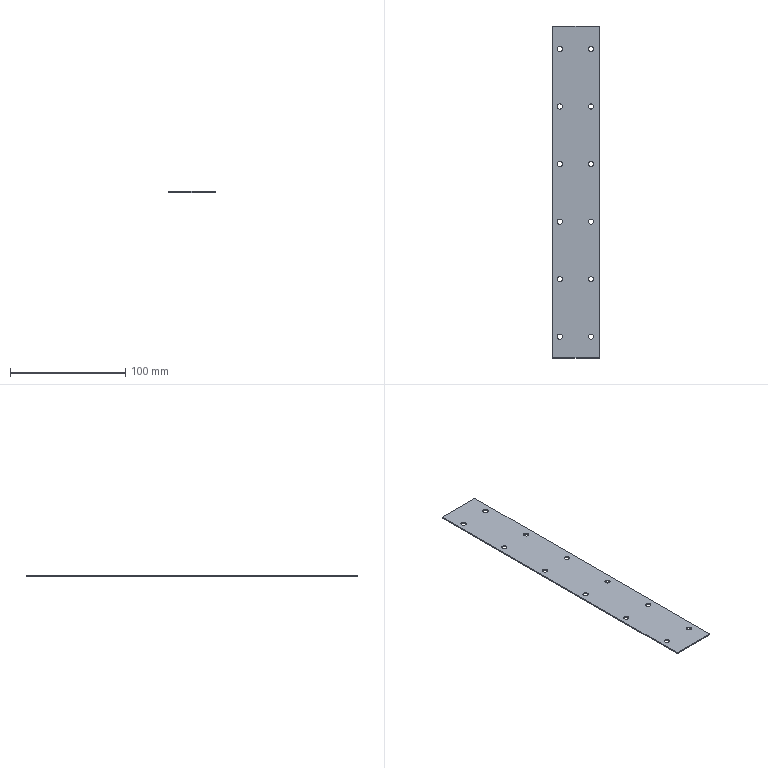Part | STEP file | Conn plate L | 1 solid | 30 faces | box 40 x 288.5 x 1 mm | volume 11349 mm3 | cylinder 24 | plane 6 | commonest cylinder face diameters 4.5 x24